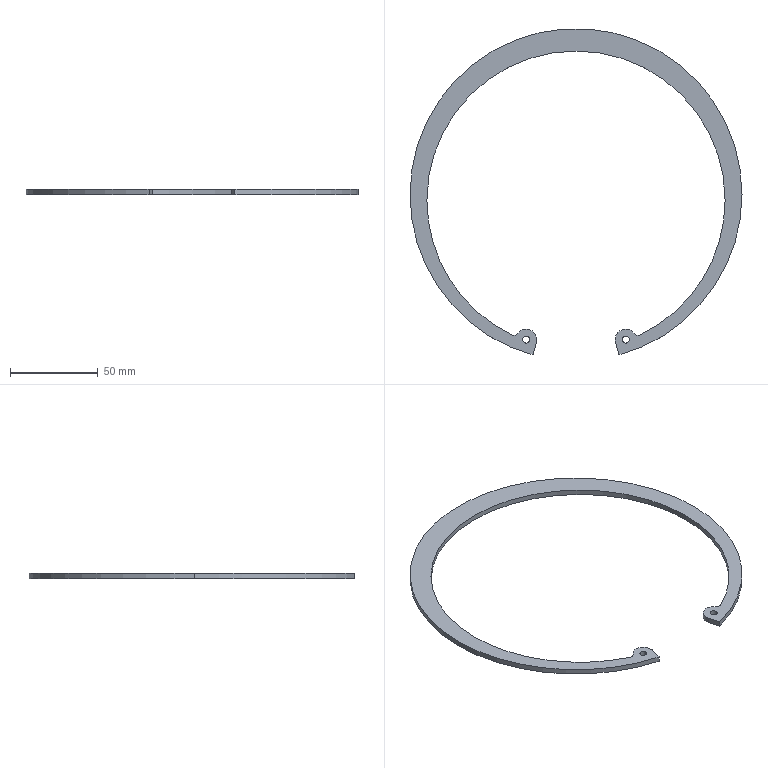Part | SolidWorks | features Extrusion 1 | 1 solid | 19 faces | box 189.5 x 186.271 x 3 mm | volume 15737 mm3 | cylinder 15 | plane 4 | commonest cylinder face diameters 4 x4 12 x3 170.2 x3 189.5 x3 6 x2
STEP:
#1=CARTESIAN_POINT('',(-30.389,-82.767,-3.));
#2=VERTEX_POINT('',#1);
#3=CARTESIAN_POINT('',(-26.389,-82.767,-3.));
#4=VERTEX_POINT('',#3);
#5=CARTESIAN_POINT('',(-28.389,-82.767,-3.));
#6=DIRECTION('',(0.,0.,1.));
#7=DIRECTION('',(1.,0.,0.));
#8=AXIS2_PLACEMENT_3D('',#5,#6,#7);
#9=CIRCLE('',#8,2.);
#10=EDGE_CURVE('',#2,#4,#9,.T.);
#11=ORIENTED_EDGE('',*,*,#10,.F.);
#12=CARTESIAN_POINT('',(-30.389,-82.767,0.));
#13=VERTEX_POINT('',#12);
#14=CARTESIAN_POINT('',(-30.389,-82.767,-3.));
#15=DIRECTION('',(0.,0.,1.));
#16=VECTOR('',#15,1000.);
#17=LINE('',#14,#16);
#18=EDGE_CURVE('',#2,#13,#17,.T.);
#19=ORIENTED_EDGE('',*,*,#18,.T.);
#20=CARTESIAN_POINT('',(-26.389,-82.767,0.));
#21=VERTEX_POINT('',#20);
#22=CARTESIAN_POINT('',(-28.389,-82.767,0.));
#23=DIRECTION('',(0.,0.,1.));
#24=DIRECTION('',(1.,0.,0.));
#25=AXIS2_PLACEMENT_3D('',#22,#23,#24);
#26=CIRCLE('',#25,2.);
#27=EDGE_CURVE('',#13,#21,#26,.T.);
#28=ORIENTED_EDGE('',*,*,#27,.T.);
#29=CARTESIAN_POINT('',(-26.389,-82.767,-3.));
#30=DIRECTION('',(0.,0.,1.));
#31=VECTOR('',#30,1000.);
#32=LINE('',#29,#31);
#33=EDGE_CURVE('',#4,#21,#32,.T.);
#34=ORIENTED_EDGE('',*,*,#33,.F.);
#35=EDGE_LOOP('',(#11,#19,#28,#34));
#36=FACE_OUTER_BOUND('',#35,.T.);
#37=CARTESIAN_POINT('',(-28.389,-82.767,-3.));
#38=DIRECTION('',(0.,0.,1.));
#39=DIRECTION('',(1.,0.,0.));
#40=AXIS2_PLACEMENT_3D('',#37,#38,#39);
#41=CYLINDRICAL_SURFACE('',#40,2.);
#42=ADVANCED_FACE('',(#36),#41,.F.);
#43=CARTESIAN_POINT('',(26.389,-82.767,-3.));
#44=VERTEX_POINT('',#43);
#45=CARTESIAN_POINT('',(30.389,-82.767,-3.));
#46=VERTEX_POINT('',#45);
#47=CARTESIAN_POINT('',(28.389,-82.767,-3.));
#48=DIRECTION('',(0.,0.,1.));
#49=DIRECTION('',(-1.,0.,0.));
#50=AXIS2_PLACEMENT_3D('',#47,#48,#49);
#51=CIRCLE('',#50,2.);
#52=EDGE_CURVE('',#44,#46,#51,.T.);
#53=ORIENTED_EDGE('',*,*,#52,.F.);
#54=CARTESIAN_POINT('',(26.389,-82.767,0.));
#55=VERTEX_POINT('',#54);
#56=CARTESIAN_POINT('',(26.389,-82.767,-3.));
#57=DIRECTION('',(0.,0.,1.));
#58=VECTOR('',#57,1000.);
#59=LINE('',#56,#58);
#60=EDGE_CURVE('',#44,#55,#59,.T.);
#61=ORIENTED_EDGE('',*,*,#60,.T.);
#62=CARTESIAN_POINT('',(30.389,-82.767,0.));
#63=VERTEX_POINT('',#62);
#64=CARTESIAN_POINT('',(28.389,-82.767,0.));
#65=DIRECTION('',(0.,0.,1.));
#66=DIRECTION('',(-1.,0.,0.));
#67=AXIS2_PLACEMENT_3D('',#64,#65,#66);
#68=CIRCLE('',#67,2.);
#69=EDGE_CURVE('',#55,#63,#68,.T.);
#70=ORIENTED_EDGE('',*,*,#69,.T.);
#71=CARTESIAN_POINT('',(30.389,-82.767,-3.));
#72=DIRECTION('',(0.,0.,1.));
#73=VECTOR('',#72,1000.);
#74=LINE('',#71,#73);
#75=EDGE_CURVE('',#46,#63,#74,.T.);
#76=ORIENTED_EDGE('',*,*,#75,.F.);
#77=EDGE_LOOP('',(#53,#61,#70,#76));
#78=FACE_OUTER_BOUND('',#77,.T.);
#79=CARTESIAN_POINT('',(28.389,-82.767,-3.));
#80=DIRECTION('',(0.,0.,1.));
#81=DIRECTION('',(1.,0.,0.));
#82=AXIS2_PLACEMENT_3D('',#79,#80,#81);
#83=CYLINDRICAL_SURFACE('',#82,2.);
#84=ADVANCED_FACE('',(#78),#83,.F.);
#85=CARTESIAN_POINT('',(-22.593,-84.32,-3.));
#86=VERTEX_POINT('',#85);
#87=CARTESIAN_POINT('',(-22.389,-82.767,-3.));
#88=VERTEX_POINT('',#87);
#89=CARTESIAN_POINT('',(-28.389,-82.767,-3.));
#90=DIRECTION('',(0.,0.,1.));
#91=DIRECTION('',(1.,0.,0.));
#92=AXIS2_PLACEMENT_3D('',#89,#90,#91);
#93=CIRCLE('',#92,6.);
#94=EDGE_CURVE('',#86,#88,#93,.T.);
#95=ORIENTED_EDGE('',*,*,#94,.T.);
#96=CARTESIAN_POINT('',(-22.389,-82.767,0.));
#97=VERTEX_POINT('',#96);
#98=CARTESIAN_POINT('',(-22.389,-82.767,-3.));
#99=DIRECTION('',(0.,0.,1.));
#100=VECTOR('',#99,1000.);
#101=LINE('',#98,#100);
#102=EDGE_CURVE('',#88,#97,#101,.T.);
#103=ORIENTED_EDGE('',*,*,#102,.T.);
#104=CARTESIAN_POINT('',(-22.593,-84.32,0.));
#105=VERTEX_POINT('',#104);
#106=CARTESIAN_POINT('',(-28.389,-82.767,0.));
#107=DIRECTION('',(0.,0.,1.));
#108=DIRECTION('',(1.,0.,0.));
#109=AXIS2_PLACEMENT_3D('',#106,#107,#108);
#110=CIRCLE('',#109,6.);
#111=EDGE_CURVE('',#105,#97,#110,.T.);
#112=ORIENTED_EDGE('',*,*,#111,.F.);
#113=CARTESIAN_POINT('',(-22.593,-84.32,-3.));
#114=DIRECTION('',(0.,0.,1.));
#115=VECTOR('',#114,1000.);
#116=LINE('',#113,#115);
#117=EDGE_CURVE('',#86,#105,#116,.T.);
#118=ORIENTED_EDGE('',*,*,#117,.F.);
#119=EDGE_LOOP('',(#95,#103,#112,#118));
#120=FACE_OUTER_BOUND('',#119,.T.);
#121=CARTESIAN_POINT('',(-28.389,-82.767,-3.));
#122=DIRECTION('',(0.,0.,1.));
#123=DIRECTION('',(1.,0.,0.));
#124=AXIS2_PLACEMENT_3D('',#121,#122,#123);
#125=CYLINDRICAL_SURFACE('',#124,6.);
#126=ADVANCED_FACE('',(#120),#125,.T.);
#127=CARTESIAN_POINT('',(-36.784,-79.939,-3.));
#128=VERTEX_POINT('',#127);
#129=CARTESIAN_POINT('',(-85.1,-3.2,-3.));
#130=VERTEX_POINT('',#129);
#131=CARTESIAN_POINT('',(0.,-3.2,-3.));
#132=DIRECTION('',(0.,0.,-1.));
#133=DIRECTION('',(1.,0.,0.));
#134=AXIS2_PLACEMENT_3D('',#131,#132,#133);
#135=CIRCLE('',#134,85.1);
#136=EDGE_CURVE('',#128,#130,#135,.T.);
#137=ORIENTED_EDGE('',*,*,#136,.T.);
#138=CARTESIAN_POINT('',(-85.1,-3.2,0.));
#139=VERTEX_POINT('',#138);
#140=CARTESIAN_POINT('',(-85.1,-3.2,-3.));
#141=DIRECTION('',(0.,0.,1.));
#142=VECTOR('',#141,1000.);
#143=LINE('',#140,#142);
#144=EDGE_CURVE('',#130,#139,#143,.T.);
#145=ORIENTED_EDGE('',*,*,#144,.T.);
#146=CARTESIAN_POINT('',(-36.784,-79.939,0.));
#147=VERTEX_POINT('',#146);
#148=CARTESIAN_POINT('',(0.,-3.2,0.));
#149=DIRECTION('',(0.,0.,-1.));
#150=DIRECTION('',(1.,0.,0.));
#151=AXIS2_PLACEMENT_3D('',#148,#149,#150);
#152=CIRCLE('',#151,85.1);
#153=EDGE_CURVE('',#147,#139,#152,.T.);
#154=ORIENTED_EDGE('',*,*,#153,.F.);
#155=CARTESIAN_POINT('',(-36.784,-79.939,-3.));
#156=DIRECTION('',(0.,0.,1.));
#157=VECTOR('',#156,1000.);
#158=LINE('',#155,#157);
#159=EDGE_CURVE('',#128,#147,#158,.T.);
#160=ORIENTED_EDGE('',*,*,#159,.F.);
#161=EDGE_LOOP('',(#137,#145,#154,#160));
#162=FACE_OUTER_BOUND('',#161,.T.);
#163=CARTESIAN_POINT('',(0.,-3.2,-3.));
#164=DIRECTION('',(0.,0.,1.));
#165=DIRECTION('',(1.,0.,0.));
#166=AXIS2_PLACEMENT_3D('',#163,#164,#165);
#167=CYLINDRICAL_SURFACE('',#166,85.1);
#168=ADVANCED_FACE('',(#162),#167,.F.);
#169=ORIENTED_EDGE('',*,*,#144,.F.);
#170=CARTESIAN_POINT('',(85.1,-3.2,-3.));
#171=VERTEX_POINT('',#170);
#172=CARTESIAN_POINT('',(0.,-3.2,-3.));
#173=DIRECTION('',(0.,0.,-1.));
#174=DIRECTION('',(1.,0.,0.));
#175=AXIS2_PLACEMENT_3D('',#172,#173,#174);
#176=CIRCLE('',#175,85.1);
#177=EDGE_CURVE('',#130,#171,#176,.T.);
#178=ORIENTED_EDGE('',*,*,#177,.T.);
#179=CARTESIAN_POINT('',(85.1,-3.2,0.));
#180=VERTEX_POINT('',#179);
#181=CARTESIAN_POINT('',(85.1,-3.2,-3.));
#182=DIRECTION('',(0.,0.,1.));
#183=VECTOR('',#182,1000.);
#184=LINE('',#181,#183);
#185=EDGE_CURVE('',#171,#180,#184,.T.);
#186=ORIENTED_EDGE('',*,*,#185,.T.);
#187=CARTESIAN_POINT('',(0.,-3.2,0.));
#188=DIRECTION('',(0.,0.,-1.));
#189=DIRECTION('',(1.,0.,0.));
#190=AXIS2_PLACEMENT_3D('',#187,#188,#189);
#191=CIRCLE('',#190,85.1);
#192=EDGE_CURVE('',#139,#180,#191,.T.);
#193=ORIENTED_EDGE('',*,*,#192,.F.);
#194=EDGE_LOOP('',(#169,#178,#186,#193));
#195=FACE_OUTER_BOUND('',#194,.T.);
#196=CARTESIAN_POINT('',(0.,-3.2,-3.));
#197=DIRECTION('',(0.,0.,1.));
#198=DIRECTION('',(1.,0.,0.));
#199=AXIS2_PLACEMENT_3D('',#196,#197,#198);
#200=CYLINDRICAL_SURFACE('',#199,85.1);
#201=ADVANCED_FACE('',(#195),#200,.F.);
#202=CARTESIAN_POINT('',(94.75,0.,-3.));
#203=VERTEX_POINT('',#202);
#204=CARTESIAN_POINT('',(-94.75,0.,-3.));
#205=VERTEX_POINT('',#204);
#206=CARTESIAN_POINT('',(0.,0.,-3.));
#207=DIRECTION('',(0.,0.,1.));
#208=DIRECTION('',(1.,0.,0.));
#209=AXIS2_PLACEMENT_3D('',#206,#207,#208);
#210=CIRCLE('',#209,94.75);
#211=EDGE_CURVE('',#203,#205,#210,.T.);
#212=ORIENTED_EDGE('',*,*,#211,.T.);
#213=CARTESIAN_POINT('',(-94.75,0.,0.));
#214=VERTEX_POINT('',#213);
#215=CARTESIAN_POINT('',(-94.75,0.,-3.));
#216=DIRECTION('',(0.,0.,1.));
#217=VECTOR('',#216,1000.);
#218=LINE('',#215,#217);
#219=EDGE_CURVE('',#205,#214,#218,.T.);
#220=ORIENTED_EDGE('',*,*,#219,.T.);
#221=CARTESIAN_POINT('',(94.75,0.,0.));
#222=VERTEX_POINT('',#221);
#223=CARTESIAN_POINT('',(0.,0.,0.));
#224=DIRECTION('',(0.,0.,1.));
#225=DIRECTION('',(1.,0.,0.));
#226=AXIS2_PLACEMENT_3D('',#223,#224,#225);
#227=CIRCLE('',#226,94.75);
#228=EDGE_CURVE('',#222,#214,#227,.T.);
#229=ORIENTED_EDGE('',*,*,#228,.F.);
#230=CARTESIAN_POINT('',(94.75,0.,-3.));
#231=DIRECTION('',(0.,0.,1.));
#232=VECTOR('',#231,1000.);
#233=LINE('',#230,#232);
#234=EDGE_CURVE('',#203,#222,#233,.T.);
#235=ORIENTED_EDGE('',*,*,#234,.F.);
#236=EDGE_LOOP('',(#212,#220,#229,#235));
#237=FACE_OUTER_BOUND('',#236,.T.);
#238=CARTESIAN_POINT('',(0.,0.,-3.));
#239=DIRECTION('',(0.,0.,1.));
#240=DIRECTION('',(1.,0.,0.));
#241=AXIS2_PLACEMENT_3D('',#238,#239,#240);
#242=CYLINDRICAL_SURFACE('',#241,94.75);
#243=ADVANCED_FACE('',(#237),#242,.T.);
#244=CARTESIAN_POINT('',(24.523,-91.521,-3.));
#245=VERTEX_POINT('',#244);
#246=CARTESIAN_POINT('',(0.,0.,-3.));
#247=DIRECTION('',(0.,0.,1.));
#248=DIRECTION('',(1.,0.,0.));
#249=AXIS2_PLACEMENT_3D('',#246,#247,#248);
#250=CIRCLE('',#249,94.75);
#251=EDGE_CURVE('',#245,#203,#250,.T.);
#252=ORIENTED_EDGE('',*,*,#251,.T.);
#253=ORIENTED_EDGE('',*,*,#234,.T.);
#254=CARTESIAN_POINT('',(24.523,-91.521,0.));
#255=VERTEX_POINT('',#254);
#256=CARTESIAN_POINT('',(0.,0.,0.));
#257=DIRECTION('',(0.,0.,1.));
#258=DIRECTION('',(1.,0.,0.));
#259=AXIS2_PLACEMENT_3D('',#256,#257,#258);
#260=CIRCLE('',#259,94.75);
#261=EDGE_CURVE('',#255,#222,#260,.T.);
#262=ORIENTED_EDGE('',*,*,#261,.F.);
#263=CARTESIAN_POINT('',(24.523,-91.521,-3.));
#264=DIRECTION('',(0.,0.,1.));
#265=VECTOR('',#264,1000.);
#266=LINE('',#263,#265);
#267=EDGE_CURVE('',#245,#255,#266,.T.);
#268=ORIENTED_EDGE('',*,*,#267,.F.);
#269=EDGE_LOOP('',(#252,#253,#262,#268));
#270=FACE_OUTER_BOUND('',#269,.T.);
#271=CARTESIAN_POINT('',(0.,0.,-3.));
#272=DIRECTION('',(0.,0.,1.));
#273=DIRECTION('',(1.,0.,0.));
#274=AXIS2_PLACEMENT_3D('',#271,#272,#273);
#275=CYLINDRICAL_SURFACE('',#274,94.75);
#276=ADVANCED_FACE('',(#270),#275,.T.);
#277=ORIENTED_EDGE('',*,*,#219,.F.);
#278=CARTESIAN_POINT('',(-24.523,-91.521,-3.));
#279=VERTEX_POINT('',#278);
#280=CARTESIAN_POINT('',(0.,0.,-3.));
#281=DIRECTION('',(0.,0.,1.));
#282=DIRECTION('',(1.,0.,0.));
#283=AXIS2_PLACEMENT_3D('',#280,#281,#282);
#284=CIRCLE('',#283,94.75);
#285=EDGE_CURVE('',#205,#279,#284,.T.);
#286=ORIENTED_EDGE('',*,*,#285,.T.);
#287=CARTESIAN_POINT('',(-24.523,-91.521,0.));
#288=VERTEX_POINT('',#287);
#289=CARTESIAN_POINT('',(-24.523,-91.521,-3.));
#290=DIRECTION('',(0.,0.,1.));
#291=VECTOR('',#290,1000.);
#292=LINE('',#289,#291);
#293=EDGE_CURVE('',#279,#288,#292,.T.);
#294=ORIENTED_EDGE('',*,*,#293,.T.);
#295=CARTESIAN_POINT('',(0.,0.,0.));
#296=DIRECTION('',(0.,0.,1.));
#297=DIRECTION('',(1.,0.,0.));
#298=AXIS2_PLACEMENT_3D('',#295,#296,#297);
#299=CIRCLE('',#298,94.75);
#300=EDGE_CURVE('',#214,#288,#299,.T.);
#301=ORIENTED_EDGE('',*,*,#300,.F.);
#302=EDGE_LOOP('',(#277,#286,#294,#301));
#303=FACE_OUTER_BOUND('',#302,.T.);
#304=CARTESIAN_POINT('',(0.,0.,-3.));
#305=DIRECTION('',(0.,0.,1.));
#306=DIRECTION('',(1.,0.,0.));
#307=AXIS2_PLACEMENT_3D('',#304,#305,#306);
#308=CYLINDRICAL_SURFACE('',#307,94.75);
#309=ADVANCED_FACE('',(#303),#308,.T.);
#310=CARTESIAN_POINT('',(22.593,-84.32,0.));
#311=VERTEX_POINT('',#310);
#312=CARTESIAN_POINT('',(22.593,-84.32,0.));
#313=DIRECTION('',(0.2588,-0.9659,0.));
#314=VECTOR('',#313,1000.);
#315=LINE('',#312,#314);
#316=EDGE_CURVE('',#311,#255,#315,.T.);
#317=ORIENTED_EDGE('',*,*,#316,.F.);
#318=CARTESIAN_POINT('',(22.593,-84.32,-3.));
#319=VERTEX_POINT('',#318);
#320=CARTESIAN_POINT('',(22.593,-84.32,-3.));
#321=DIRECTION('',(0.,0.,1.));
#322=VECTOR('',#321,1000.);
#323=LINE('',#320,#322);
#324=EDGE_CURVE('',#319,#311,#323,.T.);
#325=ORIENTED_EDGE('',*,*,#324,.F.);
#326=CARTESIAN_POINT('',(22.593,-84.32,-3.));
#327=DIRECTION('',(0.2588,-0.9659,0.));
#328=VECTOR('',#327,1000.);
#329=LINE('',#326,#328);
#330=EDGE_CURVE('',#319,#245,#329,.T.);
#331=ORIENTED_EDGE('',*,*,#330,.T.);
#332=ORIENTED_EDGE('',*,*,#267,.T.);
#333=EDGE_LOOP('',(#317,#325,#331,#332));
#334=FACE_OUTER_BOUND('',#333,.T.);
#335=CARTESIAN_POINT('',(22.593,-84.32,-3.));
#336=DIRECTION('',(-0.9659,-0.2588,0.));
#337=DIRECTION('',(0.2588,-0.9659,0.));
#338=AXIS2_PLACEMENT_3D('',#335,#336,#337);
#339=PLANE('',#338);
#340=ADVANCED_FACE('',(#334),#339,.T.);
#341=CARTESIAN_POINT('',(33.121,-79.078,0.));
#342=VERTEX_POINT('',#341);
#343=CARTESIAN_POINT('',(28.389,-82.767,0.));
#344=DIRECTION('',(0.,0.,1.));
#345=DIRECTION('',(-1.,0.,0.));
#346=AXIS2_PLACEMENT_3D('',#343,#344,#345);
#347=CIRCLE('',#346,6.);
#348=EDGE_CURVE('',#342,#311,#347,.T.);
#349=ORIENTED_EDGE('',*,*,#348,.F.);
#350=CARTESIAN_POINT('',(33.121,-79.078,-3.));
#351=VERTEX_POINT('',#350);
#352=CARTESIAN_POINT('',(33.121,-79.078,-3.));
#353=DIRECTION('',(0.,0.,1.));
#354=VECTOR('',#353,1000.);
#355=LINE('',#352,#354);
#356=EDGE_CURVE('',#351,#342,#355,.T.);
#357=ORIENTED_EDGE('',*,*,#356,.F.);
#358=CARTESIAN_POINT('',(28.389,-82.767,-3.));
#359=DIRECTION('',(0.,0.,1.));
#360=DIRECTION('',(-1.,0.,0.));
#361=AXIS2_PLACEMENT_3D('',#358,#359,#360);
#362=CIRCLE('',#361,6.);
#363=EDGE_CURVE('',#351,#319,#362,.T.);
#364=ORIENTED_EDGE('',*,*,#363,.T.);
#365=ORIENTED_EDGE('',*,*,#324,.T.);
#366=EDGE_LOOP('',(#349,#357,#364,#365));
#367=FACE_OUTER_BOUND('',#366,.T.);
#368=CARTESIAN_POINT('',(28.389,-82.767,-3.));
#369=DIRECTION('',(0.,0.,1.));
#370=DIRECTION('',(1.,0.,0.));
#371=AXIS2_PLACEMENT_3D('',#368,#369,#370);
#372=CYLINDRICAL_SURFACE('',#371,6.);
#373=ADVANCED_FACE('',(#367),#372,.T.);
#374=CARTESIAN_POINT('',(36.784,-79.939,0.));
#375=VERTEX_POINT('',#374);
#376=CARTESIAN_POINT('',(35.488,-77.234,0.));
#377=DIRECTION('',(0.,0.,-1.));
#378=DIRECTION('',(-1.,0.,0.));
#379=AXIS2_PLACEMENT_3D('',#376,#377,#378);
#380=CIRCLE('',#379,3.);
#381=EDGE_CURVE('',#375,#342,#380,.T.);
#382=ORIENTED_EDGE('',*,*,#381,.F.);
#383=CARTESIAN_POINT('',(36.784,-79.939,-3.));
#384=VERTEX_POINT('',#383);
#385=CARTESIAN_POINT('',(36.784,-79.939,-3.));
#386=DIRECTION('',(0.,0.,1.));
#387=VECTOR('',#386,1000.);
#388=LINE('',#385,#387);
#389=EDGE_CURVE('',#384,#375,#388,.T.);
#390=ORIENTED_EDGE('',*,*,#389,.F.);
#391=CARTESIAN_POINT('',(35.488,-77.234,-3.));
#392=DIRECTION('',(0.,0.,-1.));
#393=DIRECTION('',(-1.,0.,0.));
#394=AXIS2_PLACEMENT_3D('',#391,#392,#393);
#395=CIRCLE('',#394,3.);
#396=EDGE_CURVE('',#384,#351,#395,.T.);
#397=ORIENTED_EDGE('',*,*,#396,.T.);
#398=ORIENTED_EDGE('',*,*,#356,.T.);
#399=EDGE_LOOP('',(#382,#390,#397,#398));
#400=FACE_OUTER_BOUND('',#399,.T.);
#401=CARTESIAN_POINT('',(35.488,-77.234,-3.));
#402=DIRECTION('',(0.,0.,1.));
#403=DIRECTION('',(1.,0.,0.));
#404=AXIS2_PLACEMENT_3D('',#401,#402,#403);
#405=CYLINDRICAL_SURFACE('',#404,3.);
#406=ADVANCED_FACE('',(#400),#405,.F.);
#407=ORIENTED_EDGE('',*,*,#185,.F.);
#408=CARTESIAN_POINT('',(0.,-3.2,-3.));
#409=DIRECTION('',(0.,0.,-1.));
#410=DIRECTION('',(1.,0.,0.));
#411=AXIS2_PLACEMENT_3D('',#408,#409,#410);
#412=CIRCLE('',#411,85.1);
#413=EDGE_CURVE('',#171,#384,#412,.T.);
#414=ORIENTED_EDGE('',*,*,#413,.T.);
#415=ORIENTED_EDGE('',*,*,#389,.T.);
#416=CARTESIAN_POINT('',(0.,-3.2,0.));
#417=DIRECTION('',(0.,0.,-1.));
#418=DIRECTION('',(1.,0.,0.));
#419=AXIS2_PLACEMENT_3D('',#416,#417,#418);
#420=CIRCLE('',#419,85.1);
#421=EDGE_CURVE('',#180,#375,#420,.T.);
#422=ORIENTED_EDGE('',*,*,#421,.F.);
#423=EDGE_LOOP('',(#407,#414,#415,#422));
#424=FACE_OUTER_BOUND('',#423,.T.);
#425=CARTESIAN_POINT('',(0.,-3.2,-3.));
#426=DIRECTION('',(0.,0.,1.));
#427=DIRECTION('',(1.,0.,0.));
#428=AXIS2_PLACEMENT_3D('',#425,#426,#427);
#429=CYLINDRICAL_SURFACE('',#428,85.1);
#430=ADVANCED_FACE('',(#424),#429,.F.);
#431=CARTESIAN_POINT('',(-33.121,-79.078,0.));
#432=VERTEX_POINT('',#431);
#433=CARTESIAN_POINT('',(-35.488,-77.234,0.));
#434=DIRECTION('',(0.,0.,-1.));
#435=DIRECTION('',(1.,0.,0.));
#436=AXIS2_PLACEMENT_3D('',#433,#434,#435);
#437=CIRCLE('',#436,3.);
#438=EDGE_CURVE('',#432,#147,#437,.T.);
#439=ORIENTED_EDGE('',*,*,#438,.F.);
#440=CARTESIAN_POINT('',(-33.121,-79.078,-3.));
#441=VERTEX_POINT('',#440);
#442=CARTESIAN_POINT('',(-33.121,-79.078,-3.));
#443=DIRECTION('',(0.,0.,1.));
#444=VECTOR('',#443,1000.);
#445=LINE('',#442,#444);
#446=EDGE_CURVE('',#441,#432,#445,.T.);
#447=ORIENTED_EDGE('',*,*,#446,.F.);
#448=CARTESIAN_POINT('',(-35.488,-77.234,-3.));
#449=DIRECTION('',(0.,0.,-1.));
#450=DIRECTION('',(1.,0.,0.));
#451=AXIS2_PLACEMENT_3D('',#448,#449,#450);
#452=CIRCLE('',#451,3.);
#453=EDGE_CURVE('',#441,#128,#452,.T.);
#454=ORIENTED_EDGE('',*,*,#453,.T.);
#455=ORIENTED_EDGE('',*,*,#159,.T.);
#456=EDGE_LOOP('',(#439,#447,#454,#455));
#457=FACE_OUTER_BOUND('',#456,.T.);
#458=CARTESIAN_POINT('',(-35.488,-77.234,-3.));
#459=DIRECTION('',(0.,0.,1.));
#460=DIRECTION('',(1.,0.,0.));
#461=AXIS2_PLACEMENT_3D('',#458,#459,#460);
#462=CYLINDRICAL_SURFACE('',#461,3.);
#463=ADVANCED_FACE('',(#457),#462,.F.);
#464=ORIENTED_EDGE('',*,*,#102,.F.);
#465=CARTESIAN_POINT('',(-28.389,-82.767,-3.));
#466=DIRECTION('',(0.,0.,1.));
#467=DIRECTION('',(1.,0.,0.));
#468=AXIS2_PLACEMENT_3D('',#465,#466,#467);
#469=CIRCLE('',#468,6.);
#470=EDGE_CURVE('',#88,#441,#469,.T.);
#471=ORIENTED_EDGE('',*,*,#470,.T.);
#472=ORIENTED_EDGE('',*,*,#446,.T.);
#473=CARTESIAN_POINT('',(-28.389,-82.767,0.));
#474=DIRECTION('',(0.,0.,1.));
#475=DIRECTION('',(1.,0.,0.));
#476=AXIS2_PLACEMENT_3D('',#473,#474,#475);
#477=CIRCLE('',#476,6.);
#478=EDGE_CURVE('',#97,#432,#477,.T.);
#479=ORIENTED_EDGE('',*,*,#478,.F.);
#480=EDGE_LOOP('',(#464,#471,#472,#479));
#481=FACE_OUTER_BOUND('',#480,.T.);
#482=CARTESIAN_POINT('',(-28.389,-82.767,-3.));
#483=DIRECTION('',(0.,0.,1.));
#484=DIRECTION('',(1.,0.,0.));
#485=AXIS2_PLACEMENT_3D('',#482,#483,#484);
#486=CYLINDRICAL_SURFACE('',#485,6.);
#487=ADVANCED_FACE('',(#481),#486,.T.);
#488=CARTESIAN_POINT('',(-22.593,-84.32,0.));
#489=DIRECTION('',(0.2588,0.9659,0.));
#490=VECTOR('',#489,1000.);
#491=LINE('',#488,#490);
#492=EDGE_CURVE('',#288,#105,#491,.T.);
#493=ORIENTED_EDGE('',*,*,#492,.F.);
#494=ORIENTED_EDGE('',*,*,#293,.F.);
#495=CARTESIAN_POINT('',(-22.593,-84.32,-3.));
#496=DIRECTION('',(0.2588,0.9659,0.));
#497=VECTOR('',#496,1000.);
#498=LINE('',#495,#497);
#499=EDGE_CURVE('',#279,#86,#498,.T.);
#500=ORIENTED_EDGE('',*,*,#499,.T.);
#501=ORIENTED_EDGE('',*,*,#117,.T.);
#502=EDGE_LOOP('',(#493,#494,#500,#501));
#503=FACE_OUTER_BOUND('',#502,.T.);
#504=CARTESIAN_POINT('',(-22.593,-84.32,-3.));
#505=DIRECTION('',(0.9659,-0.2588,0.));
#506=DIRECTION('',(0.2588,0.9659,0.));
#507=AXIS2_PLACEMENT_3D('',#504,#505,#506);
#508=PLANE('',#507);
#509=ADVANCED_FACE('',(#503),#508,.T.);
#510=CARTESIAN_POINT('',(-28.389,-82.767,-3.));
#511=DIRECTION('',(0.,0.,1.));
#512=DIRECTION('',(1.,0.,0.));
#513=AXIS2_PLACEMENT_3D('',#510,#511,#512);
#514=CIRCLE('',#513,2.);
#515=EDGE_CURVE('',#4,#2,#514,.T.);
#516=ORIENTED_EDGE('',*,*,#515,.T.);
#517=ORIENTED_EDGE('',*,*,#10,.T.);
#518=EDGE_LOOP('',(#516,#517));
#519=FACE_BOUND('',#518,.T.);
#520=CARTESIAN_POINT('',(28.389,-82.767,-3.));
#521=DIRECTION('',(0.,0.,1.));
#522=DIRECTION('',(-1.,0.,0.));
#523=AXIS2_PLACEMENT_3D('',#520,#521,#522);
#524=CIRCLE('',#523,2.);
#525=EDGE_CURVE('',#46,#44,#524,.T.);
#526=ORIENTED_EDGE('',*,*,#525,.T.);
#527=ORIENTED_EDGE('',*,*,#52,.T.);
#528=EDGE_LOOP('',(#526,#527));
#529=FACE_BOUND('',#528,.T.);
#530=ORIENTED_EDGE('',*,*,#251,.F.);
#531=ORIENTED_EDGE('',*,*,#330,.F.);
#532=ORIENTED_EDGE('',*,*,#363,.F.);
#533=ORIENTED_EDGE('',*,*,#396,.F.);
#534=ORIENTED_EDGE('',*,*,#413,.F.);
#535=ORIENTED_EDGE('',*,*,#177,.F.);
#536=ORIENTED_EDGE('',*,*,#136,.F.);
#537=ORIENTED_EDGE('',*,*,#453,.F.);
#538=ORIENTED_EDGE('',*,*,#470,.F.);
#539=ORIENTED_EDGE('',*,*,#94,.F.);
#540=ORIENTED_EDGE('',*,*,#499,.F.);
#541=ORIENTED_EDGE('',*,*,#285,.F.);
#542=ORIENTED_EDGE('',*,*,#211,.F.);
#543=EDGE_LOOP('',(#530,#531,#532,#533,#534,#535,#536,#537,#538,#539,#540,#541,#542));
#544=FACE_OUTER_BOUND('',#543,.T.);
#545=CARTESIAN_POINT('',(0.,0.,-3.));
#546=DIRECTION('',(0.,0.,1.));
#547=DIRECTION('',(1.,0.,0.));
#548=AXIS2_PLACEMENT_3D('',#545,#546,#547);
#549=PLANE('',#548);
#550=ADVANCED_FACE('',(#519,#529,#544),#549,.F.);
#551=CARTESIAN_POINT('',(-28.389,-82.767,0.));
#552=DIRECTION('',(0.,0.,1.));
#553=DIRECTION('',(1.,0.,0.));
#554=AXIS2_PLACEMENT_3D('',#551,#552,#553);
#555=CIRCLE('',#554,2.);
#556=EDGE_CURVE('',#21,#13,#555,.T.);
#557=ORIENTED_EDGE('',*,*,#556,.F.);
#558=ORIENTED_EDGE('',*,*,#27,.F.);
#559=EDGE_LOOP('',(#557,#558));
#560=FACE_BOUND('',#559,.T.);
#561=CARTESIAN_POINT('',(28.389,-82.767,0.));
#562=DIRECTION('',(0.,0.,1.));
#563=DIRECTION('',(-1.,0.,0.));
#564=AXIS2_PLACEMENT_3D('',#561,#562,#563);
#565=CIRCLE('',#564,2.);
#566=EDGE_CURVE('',#63,#55,#565,.T.);
#567=ORIENTED_EDGE('',*,*,#566,.F.);
#568=ORIENTED_EDGE('',*,*,#69,.F.);
#569=EDGE_LOOP('',(#567,#568));
#570=FACE_BOUND('',#569,.T.);
#571=ORIENTED_EDGE('',*,*,#261,.T.);
#572=ORIENTED_EDGE('',*,*,#228,.T.);
#573=ORIENTED_EDGE('',*,*,#300,.T.);
#574=ORIENTED_EDGE('',*,*,#492,.T.);
#575=ORIENTED_EDGE('',*,*,#111,.T.);
#576=ORIENTED_EDGE('',*,*,#478,.T.);
#577=ORIENTED_EDGE('',*,*,#438,.T.);
#578=ORIENTED_EDGE('',*,*,#153,.T.);
#579=ORIENTED_EDGE('',*,*,#192,.T.);
#580=ORIENTED_EDGE('',*,*,#421,.T.);
#581=ORIENTED_EDGE('',*,*,#381,.T.);
#582=ORIENTED_EDGE('',*,*,#348,.T.);
#583=ORIENTED_EDGE('',*,*,#316,.T.);
#584=EDGE_LOOP('',(#571,#572,#573,#574,#575,#576,#577,#578,#579,#580,#581,#582,#583));
#585=FACE_OUTER_BOUND('',#584,.T.);
#586=CARTESIAN_POINT('',(0.,0.,0.));
#587=DIRECTION('',(0.,0.,1.));
#588=DIRECTION('',(1.,0.,0.));
#589=AXIS2_PLACEMENT_3D('',#586,#587,#588);
#590=PLANE('',#589);
#591=ADVANCED_FACE('',(#560,#570,#585),#590,.T.);
#592=ORIENTED_EDGE('',*,*,#60,.F.);
#593=ORIENTED_EDGE('',*,*,#525,.F.);
#594=ORIENTED_EDGE('',*,*,#75,.T.);
#595=ORIENTED_EDGE('',*,*,#566,.T.);
#596=EDGE_LOOP('',(#592,#593,#594,#595));
#597=FACE_OUTER_BOUND('',#596,.T.);
#598=CARTESIAN_POINT('',(28.389,-82.767,-3.));
#599=DIRECTION('',(0.,0.,1.));
#600=DIRECTION('',(1.,0.,0.));
#601=AXIS2_PLACEMENT_3D('',#598,#599,#600);
#602=CYLINDRICAL_SURFACE('',#601,2.);
#603=ADVANCED_FACE('',(#597),#602,.F.);
#604=ORIENTED_EDGE('',*,*,#18,.F.);
#605=ORIENTED_EDGE('',*,*,#515,.F.);
#606=ORIENTED_EDGE('',*,*,#33,.T.);
#607=ORIENTED_EDGE('',*,*,#556,.T.);
#608=EDGE_LOOP('',(#604,#605,#606,#607));
#609=FACE_OUTER_BOUND('',#608,.T.);
#610=CARTESIAN_POINT('',(-28.389,-82.767,-3.));
#611=DIRECTION('',(0.,0.,1.));
#612=DIRECTION('',(1.,0.,0.));
#613=AXIS2_PLACEMENT_3D('',#610,#611,#612);
#614=CYLINDRICAL_SURFACE('',#613,2.);
#615=ADVANCED_FACE('',(#609),#614,.F.);
#616=CLOSED_SHELL('',(#42,#84,#126,#168,#201,#243,#276,#309,#340,#373,#406,#430,#463,#487,#509,#550,#591,#603,#615));
#617=MANIFOLD_SOLID_BREP('',#616);
#618=CARTESIAN_POINT('',(0.,0.,0.));
#619=DIRECTION('',(0.,0.,1.));
#620=DIRECTION('',(1.,0.,0.));
#621=AXIS2_PLACEMENT_3D('',#618,#619,#620);
#622=(LENGTH_UNIT()NAMED_UNIT(*)SI_UNIT(.MILLI.,.METRE.));
#623=UNCERTAINTY_MEASURE_WITH_UNIT(LENGTH_MEASURE(0.00001),#622,'','');
#624=(NAMED_UNIT(*)PLANE_ANGLE_UNIT()SI_UNIT($,.RADIAN.));
#625=(NAMED_UNIT(*)SI_UNIT($,.STERADIAN.)SOLID_ANGLE_UNIT());
#626=(GEOMETRIC_REPRESENTATION_CONTEXT(3)GLOBAL_UNCERTAINTY_ASSIGNED_CONTEXT((#623))GLOBAL_UNIT_ASSIGNED_CONTEXT((#622,#624,#625))REPRESENTATION_CONTEXT('',''));
#627=ADVANCED_BREP_SHAPE_REPRESENTATION('',(#617,#621),#626);